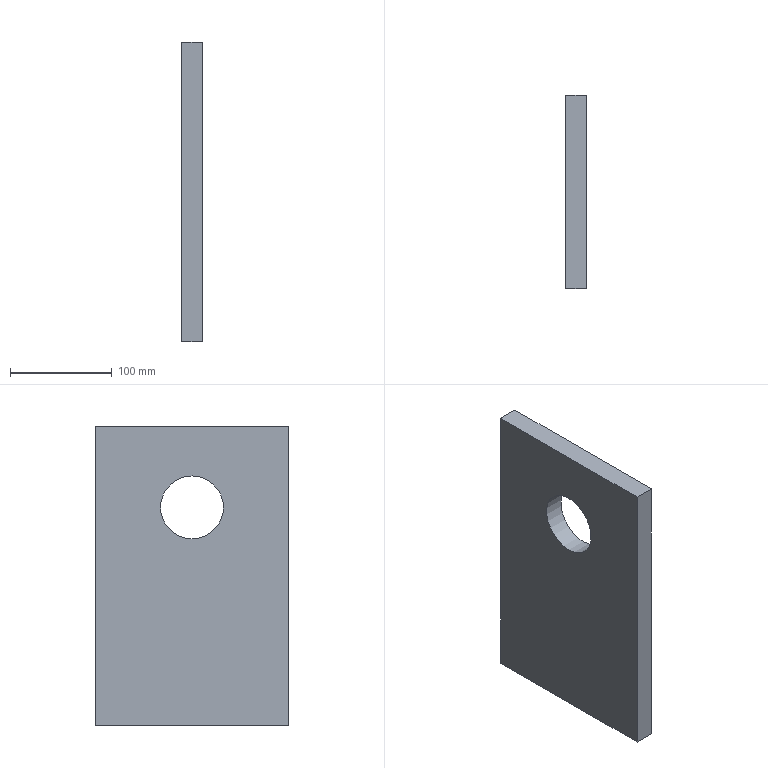Part | STEP file | Tube feed_id774_x_t | 1 solid | 7 faces | box 20 x 190 x 295 mm | volume 1060619 mm3 | plane 6 | cylinder 1 | commonest cylinder face diameters 62 x1
STEP:
#1=CARTESIAN_POINT('',(0.,0.,0.));
#2=DIRECTION('',(0.,0.,1.));
#3=DIRECTION('',(1.,0.,0.));
#4=AXIS2_PLACEMENT_3D('',#1,#2,#3);
#5=CARTESIAN_POINT('',(326.,115.936,-219.));
#6=VERTEX_POINT('',#5);
#7=CARTESIAN_POINT('',(306.,115.936,-219.));
#8=VERTEX_POINT('',#7);
#9=CARTESIAN_POINT('',(326.,115.936,-219.));
#10=DIRECTION('',(-1.,0.,0.));
#11=VECTOR('',#10,1.);
#12=LINE('',#9,#11);
#13=CARTESIAN_POINT('',(326.,115.936,-219.));
#14=DIRECTION('',(0.,0.,-1.));
#15=DIRECTION('',(0.,1.,0.));
#16=AXIS2_PLACEMENT_3D('',#13,#14,#15);
#17=PLANE('',#16);
#18=CARTESIAN_POINT('',(0.,0.));
#19=DIRECTION('',(0.,-1.));
#20=VECTOR('',#19,1.);
#21=LINE('',#18,#20);
#22=(GEOMETRIC_REPRESENTATION_CONTEXT(2)PARAMETRIC_REPRESENTATION_CONTEXT()REPRESENTATION_CONTEXT('',''));
#23=DEFINITIONAL_REPRESENTATION('',(#21),#22);
#24=PCURVE('',#17,#23);
#25=CARTESIAN_POINT('',(326.,115.936,-219.));
#26=DIRECTION('',(0.,1.,0.));
#27=DIRECTION('',(0.,0.,1.));
#28=AXIS2_PLACEMENT_3D('',#25,#26,#27);
#29=PLANE('',#28);
#30=CARTESIAN_POINT('',(0.,0.));
#31=DIRECTION('',(0.,-1.));
#32=VECTOR('',#31,1.);
#33=LINE('',#30,#32);
#34=(GEOMETRIC_REPRESENTATION_CONTEXT(2)PARAMETRIC_REPRESENTATION_CONTEXT()REPRESENTATION_CONTEXT('',''));
#35=DEFINITIONAL_REPRESENTATION('',(#33),#34);
#36=PCURVE('',#29,#35);
#37=SURFACE_CURVE('',#12,(#24,#36),.PCURVE_S1.);
#38=EDGE_CURVE('',#6,#8,#37,.T.);
#39=ORIENTED_EDGE('',*,*,#38,.T.);
#40=CARTESIAN_POINT('',(306.,305.936,-219.));
#41=VERTEX_POINT('',#40);
#42=CARTESIAN_POINT('',(306.,115.936,-219.));
#43=DIRECTION('',(0.,1.,0.));
#44=VECTOR('',#43,1.);
#45=LINE('',#42,#44);
#46=CARTESIAN_POINT('',(0.,-20.));
#47=DIRECTION('',(1.,0.));
#48=VECTOR('',#47,1.);
#49=LINE('',#46,#48);
#50=(GEOMETRIC_REPRESENTATION_CONTEXT(2)PARAMETRIC_REPRESENTATION_CONTEXT()REPRESENTATION_CONTEXT('',''));
#51=DEFINITIONAL_REPRESENTATION('',(#49),#50);
#52=PCURVE('',#17,#51);
#53=CARTESIAN_POINT('',(306.,115.936,-219.));
#54=DIRECTION('',(1.,0.,0.));
#55=DIRECTION('',(0.,0.,-1.));
#56=AXIS2_PLACEMENT_3D('',#53,#54,#55);
#57=PLANE('',#56);
#58=CARTESIAN_POINT('',(0.,0.));
#59=DIRECTION('',(0.,1.));
#60=VECTOR('',#59,1.);
#61=LINE('',#58,#60);
#62=(GEOMETRIC_REPRESENTATION_CONTEXT(2)PARAMETRIC_REPRESENTATION_CONTEXT()REPRESENTATION_CONTEXT('',''));
#63=DEFINITIONAL_REPRESENTATION('',(#61),#62);
#64=PCURVE('',#57,#63);
#65=SURFACE_CURVE('',#45,(#52,#64),.PCURVE_S1.);
#66=EDGE_CURVE('',#8,#41,#65,.T.);
#67=ORIENTED_EDGE('',*,*,#66,.T.);
#68=CARTESIAN_POINT('',(326.,305.936,-219.));
#69=VERTEX_POINT('',#68);
#70=CARTESIAN_POINT('',(326.,305.936,-219.));
#71=DIRECTION('',(-1.,0.,0.));
#72=VECTOR('',#71,1.);
#73=LINE('',#70,#72);
#74=CARTESIAN_POINT('',(190.,0.));
#75=DIRECTION('',(0.,-1.));
#76=VECTOR('',#75,1.);
#77=LINE('',#74,#76);
#78=(GEOMETRIC_REPRESENTATION_CONTEXT(2)PARAMETRIC_REPRESENTATION_CONTEXT()REPRESENTATION_CONTEXT('',''));
#79=DEFINITIONAL_REPRESENTATION('',(#77),#78);
#80=PCURVE('',#17,#79);
#81=CARTESIAN_POINT('',(326.,305.936,-219.));
#82=DIRECTION('',(0.,1.,0.));
#83=DIRECTION('',(0.,0.,1.));
#84=AXIS2_PLACEMENT_3D('',#81,#82,#83);
#85=PLANE('',#84);
#86=CARTESIAN_POINT('',(0.,0.));
#87=DIRECTION('',(0.,-1.));
#88=VECTOR('',#87,1.);
#89=LINE('',#86,#88);
#90=(GEOMETRIC_REPRESENTATION_CONTEXT(2)PARAMETRIC_REPRESENTATION_CONTEXT()REPRESENTATION_CONTEXT('',''));
#91=DEFINITIONAL_REPRESENTATION('',(#89),#90);
#92=PCURVE('',#85,#91);
#93=SURFACE_CURVE('',#73,(#80,#92),.PCURVE_S1.);
#94=EDGE_CURVE('',#69,#41,#93,.T.);
#95=ORIENTED_EDGE('',*,*,#94,.F.);
#96=CARTESIAN_POINT('',(326.,115.936,-219.));
#97=DIRECTION('',(0.,1.,0.));
#98=VECTOR('',#97,1.);
#99=LINE('',#96,#98);
#100=CARTESIAN_POINT('',(0.,0.));
#101=DIRECTION('',(1.,0.));
#102=VECTOR('',#101,1.);
#103=LINE('',#100,#102);
#104=(GEOMETRIC_REPRESENTATION_CONTEXT(2)PARAMETRIC_REPRESENTATION_CONTEXT()REPRESENTATION_CONTEXT('',''));
#105=DEFINITIONAL_REPRESENTATION('',(#103),#104);
#106=PCURVE('',#17,#105);
#107=CARTESIAN_POINT('',(326.,115.936,-219.));
#108=DIRECTION('',(1.,0.,0.));
#109=DIRECTION('',(0.,0.,-1.));
#110=AXIS2_PLACEMENT_3D('',#107,#108,#109);
#111=PLANE('',#110);
#112=CARTESIAN_POINT('',(0.,0.));
#113=DIRECTION('',(0.,1.));
#114=VECTOR('',#113,1.);
#115=LINE('',#112,#114);
#116=(GEOMETRIC_REPRESENTATION_CONTEXT(2)PARAMETRIC_REPRESENTATION_CONTEXT()REPRESENTATION_CONTEXT('',''));
#117=DEFINITIONAL_REPRESENTATION('',(#115),#116);
#118=PCURVE('',#111,#117);
#119=SURFACE_CURVE('',#99,(#106,#118),.PCURVE_S1.);
#120=EDGE_CURVE('',#6,#69,#119,.T.);
#121=ORIENTED_EDGE('',*,*,#120,.F.);
#122=EDGE_LOOP('',(#39,#67,#95,#121));
#123=FACE_BOUND('',#122,.T.);
#124=ADVANCED_FACE('',(#123),#17,.T.);
#125=ORIENTED_EDGE('',*,*,#94,.T.);
#126=CARTESIAN_POINT('',(306.,305.936,76.));
#127=VERTEX_POINT('',#126);
#128=CARTESIAN_POINT('',(306.,305.936,-219.));
#129=DIRECTION('',(0.,0.,1.));
#130=VECTOR('',#129,1.);
#131=LINE('',#128,#130);
#132=CARTESIAN_POINT('',(0.,-20.));
#133=DIRECTION('',(1.,0.));
#134=VECTOR('',#133,1.);
#135=LINE('',#132,#134);
#136=(GEOMETRIC_REPRESENTATION_CONTEXT(2)PARAMETRIC_REPRESENTATION_CONTEXT()REPRESENTATION_CONTEXT('',''));
#137=DEFINITIONAL_REPRESENTATION('',(#135),#136);
#138=PCURVE('',#85,#137);
#139=CARTESIAN_POINT('',(0.,190.));
#140=DIRECTION('',(-1.,0.));
#141=VECTOR('',#140,1.);
#142=LINE('',#139,#141);
#143=(GEOMETRIC_REPRESENTATION_CONTEXT(2)PARAMETRIC_REPRESENTATION_CONTEXT()REPRESENTATION_CONTEXT('',''));
#144=DEFINITIONAL_REPRESENTATION('',(#142),#143);
#145=PCURVE('',#57,#144);
#146=SURFACE_CURVE('',#131,(#138,#145),.PCURVE_S1.);
#147=EDGE_CURVE('',#41,#127,#146,.T.);
#148=ORIENTED_EDGE('',*,*,#147,.T.);
#149=CARTESIAN_POINT('',(326.,305.936,76.));
#150=VERTEX_POINT('',#149);
#151=CARTESIAN_POINT('',(326.,305.936,76.));
#152=DIRECTION('',(-1.,0.,0.));
#153=VECTOR('',#152,1.);
#154=LINE('',#151,#153);
#155=CARTESIAN_POINT('',(295.,0.));
#156=DIRECTION('',(0.,-1.));
#157=VECTOR('',#156,1.);
#158=LINE('',#155,#157);
#159=(GEOMETRIC_REPRESENTATION_CONTEXT(2)PARAMETRIC_REPRESENTATION_CONTEXT()REPRESENTATION_CONTEXT('',''));
#160=DEFINITIONAL_REPRESENTATION('',(#158),#159);
#161=PCURVE('',#85,#160);
#162=CARTESIAN_POINT('',(326.,115.936,76.));
#163=DIRECTION('',(0.,0.,-1.));
#164=DIRECTION('',(0.,1.,0.));
#165=AXIS2_PLACEMENT_3D('',#162,#163,#164);
#166=PLANE('',#165);
#167=CARTESIAN_POINT('',(190.,0.));
#168=DIRECTION('',(0.,-1.));
#169=VECTOR('',#168,1.);
#170=LINE('',#167,#169);
#171=(GEOMETRIC_REPRESENTATION_CONTEXT(2)PARAMETRIC_REPRESENTATION_CONTEXT()REPRESENTATION_CONTEXT('',''));
#172=DEFINITIONAL_REPRESENTATION('',(#170),#171);
#173=PCURVE('',#166,#172);
#174=SURFACE_CURVE('',#154,(#161,#173),.PCURVE_S1.);
#175=EDGE_CURVE('',#150,#127,#174,.T.);
#176=ORIENTED_EDGE('',*,*,#175,.F.);
#177=CARTESIAN_POINT('',(326.,305.936,-219.));
#178=DIRECTION('',(0.,0.,1.));
#179=VECTOR('',#178,1.);
#180=LINE('',#177,#179);
#181=CARTESIAN_POINT('',(0.,0.));
#182=DIRECTION('',(1.,0.));
#183=VECTOR('',#182,1.);
#184=LINE('',#181,#183);
#185=(GEOMETRIC_REPRESENTATION_CONTEXT(2)PARAMETRIC_REPRESENTATION_CONTEXT()REPRESENTATION_CONTEXT('',''));
#186=DEFINITIONAL_REPRESENTATION('',(#184),#185);
#187=PCURVE('',#85,#186);
#188=CARTESIAN_POINT('',(0.,190.));
#189=DIRECTION('',(-1.,0.));
#190=VECTOR('',#189,1.);
#191=LINE('',#188,#190);
#192=(GEOMETRIC_REPRESENTATION_CONTEXT(2)PARAMETRIC_REPRESENTATION_CONTEXT()REPRESENTATION_CONTEXT('',''));
#193=DEFINITIONAL_REPRESENTATION('',(#191),#192);
#194=PCURVE('',#111,#193);
#195=SURFACE_CURVE('',#180,(#187,#194),.PCURVE_S1.);
#196=EDGE_CURVE('',#69,#150,#195,.T.);
#197=ORIENTED_EDGE('',*,*,#196,.F.);
#198=EDGE_LOOP('',(#125,#148,#176,#197));
#199=FACE_BOUND('',#198,.T.);
#200=ADVANCED_FACE('',(#199),#85,.T.);
#201=ORIENTED_EDGE('',*,*,#175,.T.);
#202=CARTESIAN_POINT('',(306.,115.936,76.));
#203=VERTEX_POINT('',#202);
#204=CARTESIAN_POINT('',(306.,115.936,76.));
#205=DIRECTION('',(0.,1.,0.));
#206=VECTOR('',#205,1.);
#207=LINE('',#204,#206);
#208=CARTESIAN_POINT('',(0.,-20.));
#209=DIRECTION('',(1.,0.));
#210=VECTOR('',#209,1.);
#211=LINE('',#208,#210);
#212=(GEOMETRIC_REPRESENTATION_CONTEXT(2)PARAMETRIC_REPRESENTATION_CONTEXT()REPRESENTATION_CONTEXT('',''));
#213=DEFINITIONAL_REPRESENTATION('',(#211),#212);
#214=PCURVE('',#166,#213);
#215=CARTESIAN_POINT('',(-295.,0.));
#216=DIRECTION('',(0.,1.));
#217=VECTOR('',#216,1.);
#218=LINE('',#215,#217);
#219=(GEOMETRIC_REPRESENTATION_CONTEXT(2)PARAMETRIC_REPRESENTATION_CONTEXT()REPRESENTATION_CONTEXT('',''));
#220=DEFINITIONAL_REPRESENTATION('',(#218),#219);
#221=PCURVE('',#57,#220);
#222=SURFACE_CURVE('',#207,(#214,#221),.PCURVE_S1.);
#223=EDGE_CURVE('',#203,#127,#222,.T.);
#224=ORIENTED_EDGE('',*,*,#223,.F.);
#225=CARTESIAN_POINT('',(326.,115.936,76.));
#226=VERTEX_POINT('',#225);
#227=CARTESIAN_POINT('',(326.,115.936,76.));
#228=DIRECTION('',(-1.,0.,0.));
#229=VECTOR('',#228,1.);
#230=LINE('',#227,#229);
#231=CARTESIAN_POINT('',(0.,0.));
#232=DIRECTION('',(0.,-1.));
#233=VECTOR('',#232,1.);
#234=LINE('',#231,#233);
#235=(GEOMETRIC_REPRESENTATION_CONTEXT(2)PARAMETRIC_REPRESENTATION_CONTEXT()REPRESENTATION_CONTEXT('',''));
#236=DEFINITIONAL_REPRESENTATION('',(#234),#235);
#237=PCURVE('',#166,#236);
#238=CARTESIAN_POINT('',(295.,0.));
#239=DIRECTION('',(0.,-1.));
#240=VECTOR('',#239,1.);
#241=LINE('',#238,#240);
#242=(GEOMETRIC_REPRESENTATION_CONTEXT(2)PARAMETRIC_REPRESENTATION_CONTEXT()REPRESENTATION_CONTEXT('',''));
#243=DEFINITIONAL_REPRESENTATION('',(#241),#242);
#244=PCURVE('',#29,#243);
#245=SURFACE_CURVE('',#230,(#237,#244),.PCURVE_S1.);
#246=EDGE_CURVE('',#226,#203,#245,.T.);
#247=ORIENTED_EDGE('',*,*,#246,.F.);
#248=CARTESIAN_POINT('',(326.,115.936,76.));
#249=DIRECTION('',(0.,1.,0.));
#250=VECTOR('',#249,1.);
#251=LINE('',#248,#250);
#252=CARTESIAN_POINT('',(0.,0.));
#253=DIRECTION('',(1.,0.));
#254=VECTOR('',#253,1.);
#255=LINE('',#252,#254);
#256=(GEOMETRIC_REPRESENTATION_CONTEXT(2)PARAMETRIC_REPRESENTATION_CONTEXT()REPRESENTATION_CONTEXT('',''));
#257=DEFINITIONAL_REPRESENTATION('',(#255),#256);
#258=PCURVE('',#166,#257);
#259=CARTESIAN_POINT('',(-295.,0.));
#260=DIRECTION('',(0.,1.));
#261=VECTOR('',#260,1.);
#262=LINE('',#259,#261);
#263=(GEOMETRIC_REPRESENTATION_CONTEXT(2)PARAMETRIC_REPRESENTATION_CONTEXT()REPRESENTATION_CONTEXT('',''));
#264=DEFINITIONAL_REPRESENTATION('',(#262),#263);
#265=PCURVE('',#111,#264);
#266=SURFACE_CURVE('',#251,(#258,#265),.PCURVE_S1.);
#267=EDGE_CURVE('',#226,#150,#266,.T.);
#268=ORIENTED_EDGE('',*,*,#267,.T.);
#269=EDGE_LOOP('',(#201,#224,#247,#268));
#270=FACE_BOUND('',#269,.T.);
#271=ADVANCED_FACE('',(#270),#166,.F.);
#272=CARTESIAN_POINT('',(326.,115.936,-219.));
#273=DIRECTION('',(0.,0.,1.));
#274=VECTOR('',#273,1.);
#275=LINE('',#272,#274);
#276=CARTESIAN_POINT('',(0.,0.));
#277=DIRECTION('',(1.,0.));
#278=VECTOR('',#277,1.);
#279=LINE('',#276,#278);
#280=(GEOMETRIC_REPRESENTATION_CONTEXT(2)PARAMETRIC_REPRESENTATION_CONTEXT()REPRESENTATION_CONTEXT('',''));
#281=DEFINITIONAL_REPRESENTATION('',(#279),#280);
#282=PCURVE('',#29,#281);
#283=CARTESIAN_POINT('',(0.,0.));
#284=DIRECTION('',(-1.,0.));
#285=VECTOR('',#284,1.);
#286=LINE('',#283,#285);
#287=(GEOMETRIC_REPRESENTATION_CONTEXT(2)PARAMETRIC_REPRESENTATION_CONTEXT()REPRESENTATION_CONTEXT('',''));
#288=DEFINITIONAL_REPRESENTATION('',(#286),#287);
#289=PCURVE('',#111,#288);
#290=SURFACE_CURVE('',#275,(#282,#289),.PCURVE_S1.);
#291=EDGE_CURVE('',#6,#226,#290,.T.);
#292=ORIENTED_EDGE('',*,*,#291,.T.);
#293=ORIENTED_EDGE('',*,*,#246,.T.);
#294=CARTESIAN_POINT('',(306.,115.936,-219.));
#295=DIRECTION('',(0.,0.,1.));
#296=VECTOR('',#295,1.);
#297=LINE('',#294,#296);
#298=CARTESIAN_POINT('',(0.,-20.));
#299=DIRECTION('',(1.,0.));
#300=VECTOR('',#299,1.);
#301=LINE('',#298,#300);
#302=(GEOMETRIC_REPRESENTATION_CONTEXT(2)PARAMETRIC_REPRESENTATION_CONTEXT()REPRESENTATION_CONTEXT('',''));
#303=DEFINITIONAL_REPRESENTATION('',(#301),#302);
#304=PCURVE('',#29,#303);
#305=CARTESIAN_POINT('',(0.,0.));
#306=DIRECTION('',(-1.,0.));
#307=VECTOR('',#306,1.);
#308=LINE('',#305,#307);
#309=(GEOMETRIC_REPRESENTATION_CONTEXT(2)PARAMETRIC_REPRESENTATION_CONTEXT()REPRESENTATION_CONTEXT('',''));
#310=DEFINITIONAL_REPRESENTATION('',(#308),#309);
#311=PCURVE('',#57,#310);
#312=SURFACE_CURVE('',#297,(#304,#311),.PCURVE_S1.);
#313=EDGE_CURVE('',#8,#203,#312,.T.);
#314=ORIENTED_EDGE('',*,*,#313,.F.);
#315=ORIENTED_EDGE('',*,*,#38,.F.);
#316=EDGE_LOOP('',(#292,#293,#314,#315));
#317=FACE_BOUND('',#316,.T.);
#318=ADVANCED_FACE('',(#317),#29,.F.);
#319=CARTESIAN_POINT('',(306.,210.936,-35.));
#320=VERTEX_POINT('',#319);
#321=CARTESIAN_POINT('',(306.,210.936,-4.));
#322=DIRECTION('',(-1.,0.,0.));
#323=DIRECTION('',(0.,0.,-1.));
#324=AXIS2_PLACEMENT_3D('',#321,#322,#323);
#325=CIRCLE('',#324,31.);
#326=CARTESIAN_POINT('',(-184.,95.));
#327=CARTESIAN_POINT('',(-184.,41.306));
#328=CARTESIAN_POINT('',(-230.5,68.153));
#329=CARTESIAN_POINT('',(-277.,95.));
#330=CARTESIAN_POINT('',(-230.5,121.847));
#331=CARTESIAN_POINT('',(-184.,148.694));
#332=CARTESIAN_POINT('',(-184.,95.));
#333=(BOUNDED_CURVE()B_SPLINE_CURVE(2,(#326,#327,#328,#329,#330,#331,#332),.UNSPECIFIED.,.T.,.F.)B_SPLINE_CURVE_WITH_KNOTS((1,2,2,2,2,1),(-2.094,0.,2.094,4.189,6.283,8.378),.UNSPECIFIED.)CURVE()GEOMETRIC_REPRESENTATION_ITEM()RATIONAL_B_SPLINE_CURVE((1.,0.5,1.,0.5,1.,0.5,1.))REPRESENTATION_ITEM(''));
#334=(GEOMETRIC_REPRESENTATION_CONTEXT(2)PARAMETRIC_REPRESENTATION_CONTEXT()REPRESENTATION_CONTEXT('',''));
#335=DEFINITIONAL_REPRESENTATION('',(#333),#334);
#336=PCURVE('',#57,#335);
#337=CARTESIAN_POINT('',(375.,210.936,-4.));
#338=DIRECTION('',(-1.,0.,0.));
#339=DIRECTION('',(0.,0.,1.));
#340=AXIS2_PLACEMENT_3D('',#337,#338,#339);
#341=CYLINDRICAL_SURFACE('',#340,31.);
#342=CARTESIAN_POINT('',(3.142,69.));
#343=DIRECTION('',(1.,0.));
#344=VECTOR('',#343,1.);
#345=LINE('',#342,#344);
#346=(GEOMETRIC_REPRESENTATION_CONTEXT(2)PARAMETRIC_REPRESENTATION_CONTEXT()REPRESENTATION_CONTEXT('',''));
#347=DEFINITIONAL_REPRESENTATION('',(#345),#346);
#348=PCURVE('',#341,#347);
#349=SURFACE_CURVE('',#325,(#336,#348),.PCURVE_S1.);
#350=EDGE_CURVE('',#320,#320,#349,.T.);
#351=ORIENTED_EDGE('',*,*,#350,.F.);
#352=EDGE_LOOP('',(#351));
#353=FACE_BOUND('',#352,.T.);
#354=ORIENTED_EDGE('',*,*,#223,.T.);
#355=ORIENTED_EDGE('',*,*,#147,.F.);
#356=ORIENTED_EDGE('',*,*,#66,.F.);
#357=ORIENTED_EDGE('',*,*,#313,.T.);
#358=EDGE_LOOP('',(#354,#355,#356,#357));
#359=FACE_BOUND('',#358,.T.);
#360=ADVANCED_FACE('',(#353,#359),#57,.F.);
#361=CARTESIAN_POINT('',(326.,210.936,-35.));
#362=VERTEX_POINT('',#361);
#363=CARTESIAN_POINT('',(326.,210.936,-4.));
#364=DIRECTION('',(-1.,0.,0.));
#365=DIRECTION('',(0.,0.,-1.));
#366=AXIS2_PLACEMENT_3D('',#363,#364,#365);
#367=CIRCLE('',#366,31.);
#368=CARTESIAN_POINT('',(-184.,95.));
#369=CARTESIAN_POINT('',(-184.,41.306));
#370=CARTESIAN_POINT('',(-230.5,68.153));
#371=CARTESIAN_POINT('',(-277.,95.));
#372=CARTESIAN_POINT('',(-230.5,121.847));
#373=CARTESIAN_POINT('',(-184.,148.694));
#374=CARTESIAN_POINT('',(-184.,95.));
#375=(BOUNDED_CURVE()B_SPLINE_CURVE(2,(#368,#369,#370,#371,#372,#373,#374),.UNSPECIFIED.,.T.,.F.)B_SPLINE_CURVE_WITH_KNOTS((1,2,2,2,2,1),(-2.094,0.,2.094,4.189,6.283,8.378),.UNSPECIFIED.)CURVE()GEOMETRIC_REPRESENTATION_ITEM()RATIONAL_B_SPLINE_CURVE((1.,0.5,1.,0.5,1.,0.5,1.))REPRESENTATION_ITEM(''));
#376=(GEOMETRIC_REPRESENTATION_CONTEXT(2)PARAMETRIC_REPRESENTATION_CONTEXT()REPRESENTATION_CONTEXT('',''));
#377=DEFINITIONAL_REPRESENTATION('',(#375),#376);
#378=PCURVE('',#111,#377);
#379=CARTESIAN_POINT('',(3.142,49.));
#380=DIRECTION('',(1.,0.));
#381=VECTOR('',#380,1.);
#382=LINE('',#379,#381);
#383=(GEOMETRIC_REPRESENTATION_CONTEXT(2)PARAMETRIC_REPRESENTATION_CONTEXT()REPRESENTATION_CONTEXT('',''));
#384=DEFINITIONAL_REPRESENTATION('',(#382),#383);
#385=PCURVE('',#341,#384);
#386=SURFACE_CURVE('',#367,(#378,#385),.PCURVE_S1.);
#387=EDGE_CURVE('',#362,#362,#386,.T.);
#388=ORIENTED_EDGE('',*,*,#387,.T.);
#389=EDGE_LOOP('',(#388));
#390=FACE_BOUND('',#389,.T.);
#391=ORIENTED_EDGE('',*,*,#267,.F.);
#392=ORIENTED_EDGE('',*,*,#291,.F.);
#393=ORIENTED_EDGE('',*,*,#120,.T.);
#394=ORIENTED_EDGE('',*,*,#196,.T.);
#395=EDGE_LOOP('',(#391,#392,#393,#394));
#396=FACE_BOUND('',#395,.T.);
#397=ADVANCED_FACE('',(#390,#396),#111,.T.);
#398=ORIENTED_EDGE('',*,*,#387,.T.);
#399=CARTESIAN_POINT('',(326.,210.936,-35.));
#400=CARTESIAN_POINT('',(306.,210.936,-35.));
#401=B_SPLINE_CURVE_WITH_KNOTS('',1,(#399,#400),.UNSPECIFIED.,.F.,.F.,(2,2),(49.,69.),.PIECEWISE_BEZIER_KNOTS.);
#402=CARTESIAN_POINT('',(9.425,0.));
#403=DIRECTION('',(0.,1.));
#404=VECTOR('',#403,1.);
#405=LINE('',#402,#404);
#406=(GEOMETRIC_REPRESENTATION_CONTEXT(2)PARAMETRIC_REPRESENTATION_CONTEXT()REPRESENTATION_CONTEXT('',''));
#407=DEFINITIONAL_REPRESENTATION('',(#405),#406);
#408=PCURVE('',#341,#407);
#409=CARTESIAN_POINT('',(3.142,0.));
#410=DIRECTION('',(0.,1.));
#411=VECTOR('',#410,1.);
#412=LINE('',#409,#411);
#413=(GEOMETRIC_REPRESENTATION_CONTEXT(2)PARAMETRIC_REPRESENTATION_CONTEXT()REPRESENTATION_CONTEXT('',''));
#414=DEFINITIONAL_REPRESENTATION('',(#412),#413);
#415=PCURVE('',#341,#414);
#416=SEAM_CURVE('',#401,(#408,#415),.PCURVE_S1.);
#417=EDGE_CURVE('',#362,#320,#416,.T.);
#418=ORIENTED_EDGE('',*,*,#417,.T.);
#419=ORIENTED_EDGE('',*,*,#350,.F.);
#420=ORIENTED_EDGE('',*,*,#417,.F.);
#421=EDGE_LOOP('',(#398,#418,#419,#420));
#422=FACE_BOUND('',#421,.F.);
#423=ADVANCED_FACE('',(#422),#341,.F.);
#424=CLOSED_SHELL('',(#124,#200,#271,#318,#360,#397,#423));
#425=MANIFOLD_SOLID_BREP('',#424);
#426=(LENGTH_UNIT()NAMED_UNIT(*)SI_UNIT(.MILLI.,.METRE.));
#427=UNCERTAINTY_MEASURE_WITH_UNIT(LENGTH_MEASURE(0.000002),#426,'','');
#428=(NAMED_UNIT(*)PLANE_ANGLE_UNIT()SI_UNIT($,.RADIAN.));
#429=(NAMED_UNIT(*)SI_UNIT($,.STERADIAN.)SOLID_ANGLE_UNIT());
#430=(GEOMETRIC_REPRESENTATION_CONTEXT(3)GLOBAL_UNCERTAINTY_ASSIGNED_CONTEXT((#427))GLOBAL_UNIT_ASSIGNED_CONTEXT((#426,#428,#429))REPRESENTATION_CONTEXT('',''));
#431=ADVANCED_BREP_SHAPE_REPRESENTATION('',(#4,#425),#430);